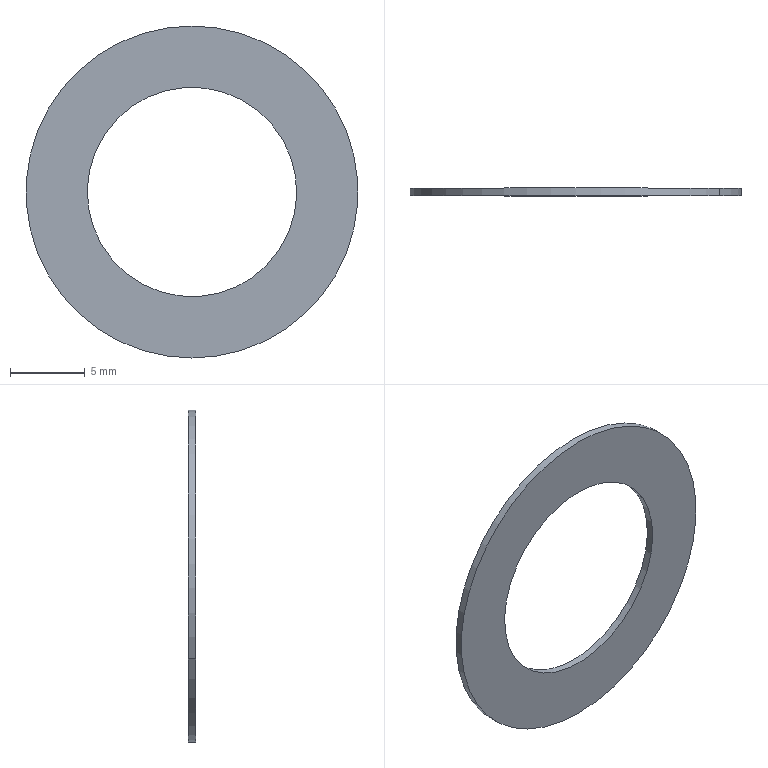Part | SolidWorks | features BaseBody 1 | 1 solid | 6 faces | box 22.2 x 0.5 x 22.2 mm | volume 116.569 mm3 | cylinder 4 | plane 2 | commonest cylinder face diameters 14 x2 22.2 x2
STEP:
#1=CARTESIAN_POINT('',(223.438,151.6,-3.5));
#2=VERTEX_POINT('',#1);
#3=CARTESIAN_POINT('',(235.562,151.6,3.5));
#4=VERTEX_POINT('',#3);
#5=CARTESIAN_POINT('',(229.5,151.6,0.));
#6=DIRECTION('',(0.,-1.,0.));
#7=DIRECTION('',(0.866,0.,0.5));
#8=AXIS2_PLACEMENT_3D('',#5,#6,#7);
#9=CIRCLE('',#8,7.);
#10=EDGE_CURVE('',#2,#4,#9,.T.);
#11=ORIENTED_EDGE('',*,*,#10,.T.);
#12=CARTESIAN_POINT('',(235.562,152.1,3.5));
#13=VERTEX_POINT('',#12);
#14=CARTESIAN_POINT('',(235.562,151.6,3.5));
#15=DIRECTION('',(0.,1.,0.));
#16=VECTOR('',#15,1000.);
#17=LINE('',#14,#16);
#18=EDGE_CURVE('',#4,#13,#17,.T.);
#19=ORIENTED_EDGE('',*,*,#18,.T.);
#20=CARTESIAN_POINT('',(223.438,152.1,-3.5));
#21=VERTEX_POINT('',#20);
#22=CARTESIAN_POINT('',(229.5,152.1,0.));
#23=DIRECTION('',(0.,-1.,0.));
#24=DIRECTION('',(0.866,0.,0.5));
#25=AXIS2_PLACEMENT_3D('',#22,#23,#24);
#26=CIRCLE('',#25,7.);
#27=EDGE_CURVE('',#21,#13,#26,.T.);
#28=ORIENTED_EDGE('',*,*,#27,.F.);
#29=CARTESIAN_POINT('',(223.438,151.6,-3.5));
#30=DIRECTION('',(0.,1.,0.));
#31=VECTOR('',#30,1000.);
#32=LINE('',#29,#31);
#33=EDGE_CURVE('',#2,#21,#32,.T.);
#34=ORIENTED_EDGE('',*,*,#33,.F.);
#35=EDGE_LOOP('',(#11,#19,#28,#34));
#36=FACE_OUTER_BOUND('',#35,.T.);
#37=CARTESIAN_POINT('',(229.5,151.6,0.));
#38=DIRECTION('',(0.,1.,0.));
#39=DIRECTION('',(-0.866,0.,-0.5));
#40=AXIS2_PLACEMENT_3D('',#37,#38,#39);
#41=CYLINDRICAL_SURFACE('',#40,7.);
#42=ADVANCED_FACE('',(#36),#41,.F.);
#43=CARTESIAN_POINT('',(239.113,151.6,5.55));
#44=VERTEX_POINT('',#43);
#45=CARTESIAN_POINT('',(219.887,151.6,-5.55));
#46=VERTEX_POINT('',#45);
#47=CARTESIAN_POINT('',(229.5,151.6,0.));
#48=DIRECTION('',(0.,-1.,0.));
#49=DIRECTION('',(0.866,0.,0.5));
#50=AXIS2_PLACEMENT_3D('',#47,#48,#49);
#51=CIRCLE('',#50,11.1);
#52=EDGE_CURVE('',#44,#46,#51,.T.);
#53=ORIENTED_EDGE('',*,*,#52,.F.);
#54=CARTESIAN_POINT('',(239.113,152.1,5.55));
#55=VERTEX_POINT('',#54);
#56=CARTESIAN_POINT('',(239.113,151.6,5.55));
#57=DIRECTION('',(0.,1.,0.));
#58=VECTOR('',#57,1000.);
#59=LINE('',#56,#58);
#60=EDGE_CURVE('',#44,#55,#59,.T.);
#61=ORIENTED_EDGE('',*,*,#60,.T.);
#62=CARTESIAN_POINT('',(219.887,152.1,-5.55));
#63=VERTEX_POINT('',#62);
#64=CARTESIAN_POINT('',(229.5,152.1,0.));
#65=DIRECTION('',(0.,-1.,0.));
#66=DIRECTION('',(0.866,0.,0.5));
#67=AXIS2_PLACEMENT_3D('',#64,#65,#66);
#68=CIRCLE('',#67,11.1);
#69=EDGE_CURVE('',#55,#63,#68,.T.);
#70=ORIENTED_EDGE('',*,*,#69,.T.);
#71=CARTESIAN_POINT('',(219.887,151.6,-5.55));
#72=DIRECTION('',(0.,1.,0.));
#73=VECTOR('',#72,1000.);
#74=LINE('',#71,#73);
#75=EDGE_CURVE('',#46,#63,#74,.T.);
#76=ORIENTED_EDGE('',*,*,#75,.F.);
#77=EDGE_LOOP('',(#53,#61,#70,#76));
#78=FACE_OUTER_BOUND('',#77,.T.);
#79=CARTESIAN_POINT('',(229.5,151.6,0.));
#80=DIRECTION('',(0.,1.,0.));
#81=DIRECTION('',(-0.866,0.,-0.5));
#82=AXIS2_PLACEMENT_3D('',#79,#80,#81);
#83=CYLINDRICAL_SURFACE('',#82,11.1);
#84=ADVANCED_FACE('',(#78),#83,.T.);
#85=CARTESIAN_POINT('',(229.5,151.6,0.));
#86=DIRECTION('',(0.,-1.,0.));
#87=DIRECTION('',(0.866,0.,0.5));
#88=AXIS2_PLACEMENT_3D('',#85,#86,#87);
#89=CIRCLE('',#88,11.1);
#90=EDGE_CURVE('',#46,#44,#89,.T.);
#91=ORIENTED_EDGE('',*,*,#90,.T.);
#92=ORIENTED_EDGE('',*,*,#52,.T.);
#93=EDGE_LOOP('',(#91,#92));
#94=FACE_OUTER_BOUND('',#93,.T.);
#95=ORIENTED_EDGE('',*,*,#10,.F.);
#96=CARTESIAN_POINT('',(229.5,151.6,0.));
#97=DIRECTION('',(0.,-1.,0.));
#98=DIRECTION('',(0.866,0.,0.5));
#99=AXIS2_PLACEMENT_3D('',#96,#97,#98);
#100=CIRCLE('',#99,7.);
#101=EDGE_CURVE('',#4,#2,#100,.T.);
#102=ORIENTED_EDGE('',*,*,#101,.F.);
#103=EDGE_LOOP('',(#95,#102));
#104=FACE_BOUND('',#103,.T.);
#105=CARTESIAN_POINT('',(229.5,151.6,0.));
#106=DIRECTION('',(0.,-1.,0.));
#107=DIRECTION('',(0.866,0.,0.5));
#108=AXIS2_PLACEMENT_3D('',#105,#106,#107);
#109=PLANE('',#108);
#110=ADVANCED_FACE('',(#94,#104),#109,.T.);
#111=CARTESIAN_POINT('',(229.5,152.1,0.));
#112=DIRECTION('',(0.,-1.,0.));
#113=DIRECTION('',(0.866,0.,0.5));
#114=AXIS2_PLACEMENT_3D('',#111,#112,#113);
#115=CIRCLE('',#114,11.1);
#116=EDGE_CURVE('',#63,#55,#115,.T.);
#117=ORIENTED_EDGE('',*,*,#116,.F.);
#118=ORIENTED_EDGE('',*,*,#69,.F.);
#119=EDGE_LOOP('',(#117,#118));
#120=FACE_OUTER_BOUND('',#119,.T.);
#121=ORIENTED_EDGE('',*,*,#27,.T.);
#122=CARTESIAN_POINT('',(229.5,152.1,0.));
#123=DIRECTION('',(0.,-1.,0.));
#124=DIRECTION('',(0.866,0.,0.5));
#125=AXIS2_PLACEMENT_3D('',#122,#123,#124);
#126=CIRCLE('',#125,7.);
#127=EDGE_CURVE('',#13,#21,#126,.T.);
#128=ORIENTED_EDGE('',*,*,#127,.T.);
#129=EDGE_LOOP('',(#121,#128));
#130=FACE_BOUND('',#129,.T.);
#131=CARTESIAN_POINT('',(229.5,152.1,0.));
#132=DIRECTION('',(0.,-1.,0.));
#133=DIRECTION('',(0.866,0.,0.5));
#134=AXIS2_PLACEMENT_3D('',#131,#132,#133);
#135=PLANE('',#134);
#136=ADVANCED_FACE('',(#120,#130),#135,.F.);
#137=ORIENTED_EDGE('',*,*,#60,.F.);
#138=ORIENTED_EDGE('',*,*,#90,.F.);
#139=ORIENTED_EDGE('',*,*,#75,.T.);
#140=ORIENTED_EDGE('',*,*,#116,.T.);
#141=EDGE_LOOP('',(#137,#138,#139,#140));
#142=FACE_OUTER_BOUND('',#141,.T.);
#143=CARTESIAN_POINT('',(229.5,151.6,0.));
#144=DIRECTION('',(0.,1.,0.));
#145=DIRECTION('',(-0.866,0.,-0.5));
#146=AXIS2_PLACEMENT_3D('',#143,#144,#145);
#147=CYLINDRICAL_SURFACE('',#146,11.1);
#148=ADVANCED_FACE('',(#142),#147,.T.);
#149=ORIENTED_EDGE('',*,*,#18,.F.);
#150=ORIENTED_EDGE('',*,*,#101,.T.);
#151=ORIENTED_EDGE('',*,*,#33,.T.);
#152=ORIENTED_EDGE('',*,*,#127,.F.);
#153=EDGE_LOOP('',(#149,#150,#151,#152));
#154=FACE_OUTER_BOUND('',#153,.T.);
#155=CARTESIAN_POINT('',(229.5,151.6,0.));
#156=DIRECTION('',(0.,1.,0.));
#157=DIRECTION('',(-0.866,0.,-0.5));
#158=AXIS2_PLACEMENT_3D('',#155,#156,#157);
#159=CYLINDRICAL_SURFACE('',#158,7.);
#160=ADVANCED_FACE('',(#154),#159,.F.);
#161=CLOSED_SHELL('',(#42,#84,#110,#136,#148,#160));
#162=MANIFOLD_SOLID_BREP('',#161);
#163=CARTESIAN_POINT('',(0.,0.,0.));
#164=DIRECTION('',(0.,0.,1.));
#165=DIRECTION('',(1.,0.,0.));
#166=AXIS2_PLACEMENT_3D('',#163,#164,#165);
#167=(LENGTH_UNIT()NAMED_UNIT(*)SI_UNIT(.MILLI.,.METRE.));
#168=UNCERTAINTY_MEASURE_WITH_UNIT(LENGTH_MEASURE(0.00001),#167,'','');
#169=(NAMED_UNIT(*)PLANE_ANGLE_UNIT()SI_UNIT($,.RADIAN.));
#170=(NAMED_UNIT(*)SI_UNIT($,.STERADIAN.)SOLID_ANGLE_UNIT());
#171=(GEOMETRIC_REPRESENTATION_CONTEXT(3)GLOBAL_UNCERTAINTY_ASSIGNED_CONTEXT((#168))GLOBAL_UNIT_ASSIGNED_CONTEXT((#167,#169,#170))REPRESENTATION_CONTEXT('',''));
#172=ADVANCED_BREP_SHAPE_REPRESENTATION('',(#162,#166),#171);